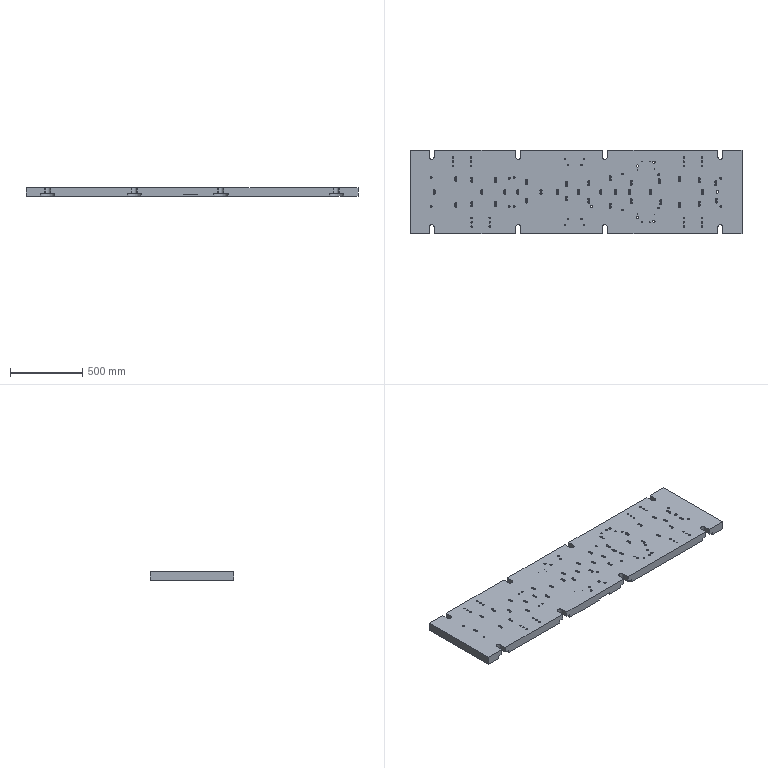Part | NX | features UP-1 2 | 1 solid | 815 faces | box 2300 x 580 x 60 mm | volume 72022458 mm3 | cylinder 406 | plane 255 | cone 154 | commonest cylinder face diameters 10 x75 9 x72 14.5 x72 8.5 x38 52.004 x34 10.506 x24